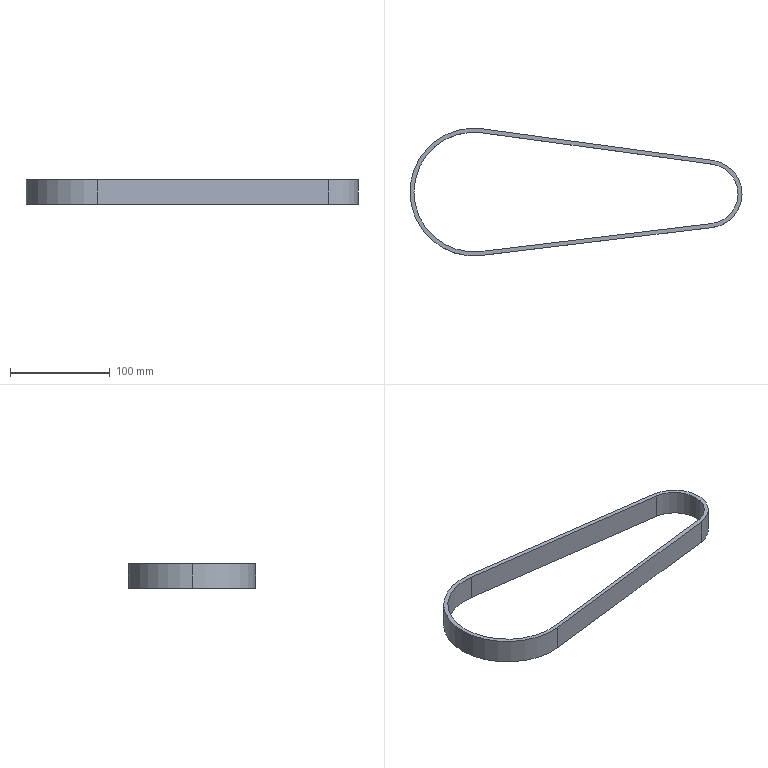Part | STEP file | Drive belt | 1 solid | 12 faces | box 332.993 x 128 x 25 mm | volume 76914 mm3 | cylinder 6 | plane 6 | commonest cylinder face diameters 120 x2 128 x2 60 x1 68 x1
STEP:
#1=CARTESIAN_POINT('',(-114.273,11.253,25.));
#2=VERTEX_POINT('',#1);
#3=CARTESIAN_POINT('',(-46.154,70.702,25.));
#4=VERTEX_POINT('',#3);
#5=CARTESIAN_POINT('',(-54.273,11.253,25.));
#6=DIRECTION('',(0.,0.,-1.));
#7=DIRECTION('',(-1.,0.,0.));
#8=AXIS2_PLACEMENT_3D('',#5,#6,#7);
#9=CIRCLE('',#8,60.);
#10=EDGE_CURVE('',#2,#4,#9,.T.);
#11=ORIENTED_EDGE('',*,*,#10,.F.);
#12=CARTESIAN_POINT('',(-114.273,11.253,0.));
#13=VERTEX_POINT('',#12);
#14=CARTESIAN_POINT('',(-114.273,11.253,25.));
#15=DIRECTION('',(0.,0.,-1.));
#16=VECTOR('',#15,1000.);
#17=LINE('',#14,#16);
#18=EDGE_CURVE('',#2,#13,#17,.T.);
#19=ORIENTED_EDGE('',*,*,#18,.T.);
#20=CARTESIAN_POINT('',(-46.154,70.702,0.));
#21=VERTEX_POINT('',#20);
#22=CARTESIAN_POINT('',(-54.273,11.253,0.));
#23=DIRECTION('',(0.,0.,1.));
#24=DIRECTION('',(-1.,0.,0.));
#25=AXIS2_PLACEMENT_3D('',#22,#23,#24);
#26=CIRCLE('',#25,60.);
#27=EDGE_CURVE('',#21,#13,#26,.T.);
#28=ORIENTED_EDGE('',*,*,#27,.F.);
#29=CARTESIAN_POINT('',(-46.154,70.702,25.));
#30=DIRECTION('',(0.,0.,-1.));
#31=VECTOR('',#30,1000.);
#32=LINE('',#29,#31);
#33=EDGE_CURVE('',#4,#21,#32,.T.);
#34=ORIENTED_EDGE('',*,*,#33,.F.);
#35=EDGE_LOOP('',(#11,#19,#28,#34));
#36=FACE_OUTER_BOUND('',#35,.T.);
#37=CARTESIAN_POINT('',(-54.273,11.253,25.));
#38=DIRECTION('',(0.,0.,-1.));
#39=DIRECTION('',(-1.,0.,0.));
#40=AXIS2_PLACEMENT_3D('',#37,#38,#39);
#41=CYLINDRICAL_SURFACE('',#40,60.);
#42=ADVANCED_FACE('',(#36),#41,.F.);
#43=CARTESIAN_POINT('',(-118.273,11.253,25.));
#44=VERTEX_POINT('',#43);
#45=CARTESIAN_POINT('',(-46.593,-52.284,25.));
#46=VERTEX_POINT('',#45);
#47=CARTESIAN_POINT('',(-54.273,11.253,25.));
#48=DIRECTION('',(0.,0.,1.));
#49=DIRECTION('',(-1.,0.,0.));
#50=AXIS2_PLACEMENT_3D('',#47,#48,#49);
#51=CIRCLE('',#50,64.);
#52=EDGE_CURVE('',#44,#46,#51,.T.);
#53=ORIENTED_EDGE('',*,*,#52,.F.);
#54=CARTESIAN_POINT('',(-118.273,11.253,0.));
#55=VERTEX_POINT('',#54);
#56=CARTESIAN_POINT('',(-118.273,11.253,25.));
#57=DIRECTION('',(0.,0.,-1.));
#58=VECTOR('',#57,1000.);
#59=LINE('',#56,#58);
#60=EDGE_CURVE('',#44,#55,#59,.T.);
#61=ORIENTED_EDGE('',*,*,#60,.T.);
#62=CARTESIAN_POINT('',(-46.593,-52.284,0.));
#63=VERTEX_POINT('',#62);
#64=CARTESIAN_POINT('',(-54.273,11.253,0.));
#65=DIRECTION('',(0.,0.,1.));
#66=DIRECTION('',(-1.,0.,0.));
#67=AXIS2_PLACEMENT_3D('',#64,#65,#66);
#68=CIRCLE('',#67,64.);
#69=EDGE_CURVE('',#55,#63,#68,.T.);
#70=ORIENTED_EDGE('',*,*,#69,.T.);
#71=CARTESIAN_POINT('',(-46.593,-52.284,25.));
#72=DIRECTION('',(0.,0.,1.));
#73=VECTOR('',#72,1000.);
#74=LINE('',#71,#73);
#75=EDGE_CURVE('',#63,#46,#74,.T.);
#76=ORIENTED_EDGE('',*,*,#75,.T.);
#77=EDGE_LOOP('',(#53,#61,#70,#76));
#78=FACE_OUTER_BOUND('',#77,.T.);
#79=CARTESIAN_POINT('',(-54.273,11.253,25.));
#80=DIRECTION('',(0.,0.,-1.));
#81=DIRECTION('',(-1.,0.,0.));
#82=AXIS2_PLACEMENT_3D('',#79,#80,#81);
#83=CYLINDRICAL_SURFACE('',#82,64.);
#84=ADVANCED_FACE('',(#78),#83,.T.);
#85=CARTESIAN_POINT('',(184.78,39.164,25.));
#86=VERTEX_POINT('',#85);
#87=CARTESIAN_POINT('',(-46.154,70.702,25.));
#88=DIRECTION('',(-0.9908,0.1353,0.));
#89=VECTOR('',#88,1000.);
#90=LINE('',#87,#89);
#91=EDGE_CURVE('',#86,#4,#90,.T.);
#92=ORIENTED_EDGE('',*,*,#91,.T.);
#93=ORIENTED_EDGE('',*,*,#33,.T.);
#94=CARTESIAN_POINT('',(184.78,39.164,0.));
#95=VERTEX_POINT('',#94);
#96=CARTESIAN_POINT('',(-46.154,70.702,0.));
#97=DIRECTION('',(0.9908,-0.1353,0.));
#98=VECTOR('',#97,1000.);
#99=LINE('',#96,#98);
#100=EDGE_CURVE('',#21,#95,#99,.T.);
#101=ORIENTED_EDGE('',*,*,#100,.T.);
#102=CARTESIAN_POINT('',(184.78,39.164,25.));
#103=DIRECTION('',(0.,0.,1.));
#104=VECTOR('',#103,1000.);
#105=LINE('',#102,#104);
#106=EDGE_CURVE('',#95,#86,#105,.T.);
#107=ORIENTED_EDGE('',*,*,#106,.T.);
#108=EDGE_LOOP('',(#92,#93,#101,#107));
#109=FACE_OUTER_BOUND('',#108,.T.);
#110=CARTESIAN_POINT('',(-46.154,70.702,25.));
#111=DIRECTION('',(-0.1353,-0.9908,0.));
#112=DIRECTION('',(0.9908,-0.1353,0.));
#113=AXIS2_PLACEMENT_3D('',#110,#111,#112);
#114=PLANE('',#113);
#115=ADVANCED_FACE('',(#109),#114,.T.);
#116=ORIENTED_EDGE('',*,*,#18,.F.);
#117=CARTESIAN_POINT('',(-47.073,-48.313,25.));
#118=VERTEX_POINT('',#117);
#119=CARTESIAN_POINT('',(-54.273,11.253,25.));
#120=DIRECTION('',(0.,0.,-1.));
#121=DIRECTION('',(-1.,0.,0.));
#122=AXIS2_PLACEMENT_3D('',#119,#120,#121);
#123=CIRCLE('',#122,60.);
#124=EDGE_CURVE('',#118,#2,#123,.T.);
#125=ORIENTED_EDGE('',*,*,#124,.F.);
#126=CARTESIAN_POINT('',(-47.073,-48.313,0.));
#127=VERTEX_POINT('',#126);
#128=CARTESIAN_POINT('',(-47.073,-48.313,25.));
#129=DIRECTION('',(0.,0.,1.));
#130=VECTOR('',#129,1000.);
#131=LINE('',#128,#130);
#132=EDGE_CURVE('',#127,#118,#131,.T.);
#133=ORIENTED_EDGE('',*,*,#132,.F.);
#134=CARTESIAN_POINT('',(-54.273,11.253,0.));
#135=DIRECTION('',(0.,0.,1.));
#136=DIRECTION('',(-1.,0.,0.));
#137=AXIS2_PLACEMENT_3D('',#134,#135,#136);
#138=CIRCLE('',#137,60.);
#139=EDGE_CURVE('',#13,#127,#138,.T.);
#140=ORIENTED_EDGE('',*,*,#139,.F.);
#141=EDGE_LOOP('',(#116,#125,#133,#140));
#142=FACE_OUTER_BOUND('',#141,.T.);
#143=CARTESIAN_POINT('',(-54.273,11.253,25.));
#144=DIRECTION('',(0.,0.,-1.));
#145=DIRECTION('',(-1.,0.,0.));
#146=AXIS2_PLACEMENT_3D('',#143,#144,#145);
#147=CYLINDRICAL_SURFACE('',#146,60.);
#148=ADVANCED_FACE('',(#142),#147,.F.);
#149=ORIENTED_EDGE('',*,*,#91,.F.);
#150=CARTESIAN_POINT('',(184.32,-20.344,25.));
#151=VERTEX_POINT('',#150);
#152=CARTESIAN_POINT('',(180.72,9.439,25.));
#153=DIRECTION('',(0.,0.,-1.));
#154=DIRECTION('',(-1.,0.,0.));
#155=AXIS2_PLACEMENT_3D('',#152,#153,#154);
#156=CIRCLE('',#155,30.);
#157=EDGE_CURVE('',#86,#151,#156,.T.);
#158=ORIENTED_EDGE('',*,*,#157,.T.);
#159=CARTESIAN_POINT('',(184.32,-20.344,25.));
#160=DIRECTION('',(-0.9928,-0.12,0.));
#161=VECTOR('',#160,1000.);
#162=LINE('',#159,#161);
#163=EDGE_CURVE('',#151,#118,#162,.T.);
#164=ORIENTED_EDGE('',*,*,#163,.T.);
#165=ORIENTED_EDGE('',*,*,#124,.T.);
#166=ORIENTED_EDGE('',*,*,#10,.T.);
#167=EDGE_LOOP('',(#149,#158,#164,#165,#166));
#168=FACE_BOUND('',#167,.T.);
#169=CARTESIAN_POINT('',(-45.613,74.665,25.));
#170=VERTEX_POINT('',#169);
#171=CARTESIAN_POINT('',(-54.273,11.253,25.));
#172=DIRECTION('',(0.,0.,1.));
#173=DIRECTION('',(-1.,0.,0.));
#174=AXIS2_PLACEMENT_3D('',#171,#172,#173);
#175=CIRCLE('',#174,64.);
#176=EDGE_CURVE('',#170,#44,#175,.T.);
#177=ORIENTED_EDGE('',*,*,#176,.T.);
#178=ORIENTED_EDGE('',*,*,#52,.T.);
#179=CARTESIAN_POINT('',(184.8,-24.315,25.));
#180=VERTEX_POINT('',#179);
#181=CARTESIAN_POINT('',(-46.593,-52.284,25.));
#182=DIRECTION('',(0.9928,0.12,0.));
#183=VECTOR('',#182,1000.);
#184=LINE('',#181,#183);
#185=EDGE_CURVE('',#46,#180,#184,.T.);
#186=ORIENTED_EDGE('',*,*,#185,.T.);
#187=CARTESIAN_POINT('',(185.321,43.127,25.));
#188=VERTEX_POINT('',#187);
#189=CARTESIAN_POINT('',(180.72,9.439,25.));
#190=DIRECTION('',(0.,0.,1.));
#191=DIRECTION('',(-1.,0.,0.));
#192=AXIS2_PLACEMENT_3D('',#189,#190,#191);
#193=CIRCLE('',#192,34.);
#194=EDGE_CURVE('',#180,#188,#193,.T.);
#195=ORIENTED_EDGE('',*,*,#194,.T.);
#196=CARTESIAN_POINT('',(185.321,43.127,25.));
#197=DIRECTION('',(-0.9908,0.1353,0.));
#198=VECTOR('',#197,1000.);
#199=LINE('',#196,#198);
#200=EDGE_CURVE('',#188,#170,#199,.T.);
#201=ORIENTED_EDGE('',*,*,#200,.T.);
#202=EDGE_LOOP('',(#177,#178,#186,#195,#201));
#203=FACE_OUTER_BOUND('',#202,.T.);
#204=CARTESIAN_POINT('',(180.72,9.439,25.));
#205=DIRECTION('',(0.,0.,1.));
#206=DIRECTION('',(1.,0.,0.));
#207=AXIS2_PLACEMENT_3D('',#204,#205,#206);
#208=PLANE('',#207);
#209=ADVANCED_FACE('',(#168,#203),#208,.T.);
#210=CARTESIAN_POINT('',(184.32,-20.344,0.));
#211=VERTEX_POINT('',#210);
#212=CARTESIAN_POINT('',(184.32,-20.344,25.));
#213=DIRECTION('',(0.,0.,-1.));
#214=VECTOR('',#213,1000.);
#215=LINE('',#212,#214);
#216=EDGE_CURVE('',#151,#211,#215,.T.);
#217=ORIENTED_EDGE('',*,*,#216,.F.);
#218=ORIENTED_EDGE('',*,*,#157,.F.);
#219=ORIENTED_EDGE('',*,*,#106,.F.);
#220=CARTESIAN_POINT('',(180.72,9.439,0.));
#221=DIRECTION('',(0.,0.,1.));
#222=DIRECTION('',(-1.,0.,0.));
#223=AXIS2_PLACEMENT_3D('',#220,#221,#222);
#224=CIRCLE('',#223,30.);
#225=EDGE_CURVE('',#211,#95,#224,.T.);
#226=ORIENTED_EDGE('',*,*,#225,.F.);
#227=EDGE_LOOP('',(#217,#218,#219,#226));
#228=FACE_OUTER_BOUND('',#227,.T.);
#229=CARTESIAN_POINT('',(180.72,9.439,25.));
#230=DIRECTION('',(0.,0.,-1.));
#231=DIRECTION('',(-1.,0.,0.));
#232=AXIS2_PLACEMENT_3D('',#229,#230,#231);
#233=CYLINDRICAL_SURFACE('',#232,30.);
#234=ADVANCED_FACE('',(#228),#233,.F.);
#235=ORIENTED_EDGE('',*,*,#27,.T.);
#236=ORIENTED_EDGE('',*,*,#139,.T.);
#237=CARTESIAN_POINT('',(184.32,-20.344,0.));
#238=DIRECTION('',(-0.9928,-0.12,0.));
#239=VECTOR('',#238,1000.);
#240=LINE('',#237,#239);
#241=EDGE_CURVE('',#211,#127,#240,.T.);
#242=ORIENTED_EDGE('',*,*,#241,.F.);
#243=ORIENTED_EDGE('',*,*,#225,.T.);
#244=ORIENTED_EDGE('',*,*,#100,.F.);
#245=EDGE_LOOP('',(#235,#236,#242,#243,#244));
#246=FACE_BOUND('',#245,.T.);
#247=CARTESIAN_POINT('',(184.8,-24.315,0.));
#248=VERTEX_POINT('',#247);
#249=CARTESIAN_POINT('',(-46.593,-52.284,0.));
#250=DIRECTION('',(0.9928,0.12,0.));
#251=VECTOR('',#250,1000.);
#252=LINE('',#249,#251);
#253=EDGE_CURVE('',#63,#248,#252,.T.);
#254=ORIENTED_EDGE('',*,*,#253,.F.);
#255=ORIENTED_EDGE('',*,*,#69,.F.);
#256=CARTESIAN_POINT('',(-45.613,74.665,0.));
#257=VERTEX_POINT('',#256);
#258=CARTESIAN_POINT('',(-54.273,11.253,0.));
#259=DIRECTION('',(0.,0.,1.));
#260=DIRECTION('',(-1.,0.,0.));
#261=AXIS2_PLACEMENT_3D('',#258,#259,#260);
#262=CIRCLE('',#261,64.);
#263=EDGE_CURVE('',#257,#55,#262,.T.);
#264=ORIENTED_EDGE('',*,*,#263,.F.);
#265=CARTESIAN_POINT('',(185.321,43.127,0.));
#266=VERTEX_POINT('',#265);
#267=CARTESIAN_POINT('',(185.321,43.127,0.));
#268=DIRECTION('',(-0.9908,0.1353,0.));
#269=VECTOR('',#268,1000.);
#270=LINE('',#267,#269);
#271=EDGE_CURVE('',#266,#257,#270,.T.);
#272=ORIENTED_EDGE('',*,*,#271,.F.);
#273=CARTESIAN_POINT('',(180.72,9.439,0.));
#274=DIRECTION('',(0.,0.,1.));
#275=DIRECTION('',(-1.,0.,0.));
#276=AXIS2_PLACEMENT_3D('',#273,#274,#275);
#277=CIRCLE('',#276,34.);
#278=EDGE_CURVE('',#248,#266,#277,.T.);
#279=ORIENTED_EDGE('',*,*,#278,.F.);
#280=EDGE_LOOP('',(#254,#255,#264,#272,#279));
#281=FACE_OUTER_BOUND('',#280,.T.);
#282=CARTESIAN_POINT('',(180.72,9.439,0.));
#283=DIRECTION('',(0.,0.,1.));
#284=DIRECTION('',(1.,0.,0.));
#285=AXIS2_PLACEMENT_3D('',#282,#283,#284);
#286=PLANE('',#285);
#287=ADVANCED_FACE('',(#246,#281),#286,.F.);
#288=ORIENTED_EDGE('',*,*,#163,.F.);
#289=ORIENTED_EDGE('',*,*,#216,.T.);
#290=ORIENTED_EDGE('',*,*,#241,.T.);
#291=ORIENTED_EDGE('',*,*,#132,.T.);
#292=EDGE_LOOP('',(#288,#289,#290,#291));
#293=FACE_OUTER_BOUND('',#292,.T.);
#294=CARTESIAN_POINT('',(-47.073,-48.313,25.));
#295=DIRECTION('',(-0.12,0.9928,0.));
#296=DIRECTION('',(-0.9928,-0.12,0.));
#297=AXIS2_PLACEMENT_3D('',#294,#295,#296);
#298=PLANE('',#297);
#299=ADVANCED_FACE('',(#293),#298,.T.);
#300=CARTESIAN_POINT('',(184.8,-24.315,25.));
#301=DIRECTION('',(0.,0.,-1.));
#302=VECTOR('',#301,1000.);
#303=LINE('',#300,#302);
#304=EDGE_CURVE('',#180,#248,#303,.T.);
#305=ORIENTED_EDGE('',*,*,#304,.F.);
#306=ORIENTED_EDGE('',*,*,#185,.F.);
#307=ORIENTED_EDGE('',*,*,#75,.F.);
#308=ORIENTED_EDGE('',*,*,#253,.T.);
#309=EDGE_LOOP('',(#305,#306,#307,#308));
#310=FACE_OUTER_BOUND('',#309,.T.);
#311=CARTESIAN_POINT('',(-46.593,-52.284,25.));
#312=DIRECTION('',(-0.12,0.9928,0.));
#313=DIRECTION('',(-0.9928,-0.12,0.));
#314=AXIS2_PLACEMENT_3D('',#311,#312,#313);
#315=PLANE('',#314);
#316=ADVANCED_FACE('',(#310),#315,.F.);
#317=ORIENTED_EDGE('',*,*,#60,.F.);
#318=ORIENTED_EDGE('',*,*,#176,.F.);
#319=CARTESIAN_POINT('',(-45.613,74.665,25.));
#320=DIRECTION('',(0.,0.,-1.));
#321=VECTOR('',#320,1000.);
#322=LINE('',#319,#321);
#323=EDGE_CURVE('',#170,#257,#322,.T.);
#324=ORIENTED_EDGE('',*,*,#323,.T.);
#325=ORIENTED_EDGE('',*,*,#263,.T.);
#326=EDGE_LOOP('',(#317,#318,#324,#325));
#327=FACE_OUTER_BOUND('',#326,.T.);
#328=CARTESIAN_POINT('',(-54.273,11.253,25.));
#329=DIRECTION('',(0.,0.,-1.));
#330=DIRECTION('',(-1.,0.,0.));
#331=AXIS2_PLACEMENT_3D('',#328,#329,#330);
#332=CYLINDRICAL_SURFACE('',#331,64.);
#333=ADVANCED_FACE('',(#327),#332,.T.);
#334=ORIENTED_EDGE('',*,*,#323,.F.);
#335=ORIENTED_EDGE('',*,*,#200,.F.);
#336=CARTESIAN_POINT('',(185.321,43.127,25.));
#337=DIRECTION('',(0.,0.,1.));
#338=VECTOR('',#337,1000.);
#339=LINE('',#336,#338);
#340=EDGE_CURVE('',#266,#188,#339,.T.);
#341=ORIENTED_EDGE('',*,*,#340,.F.);
#342=ORIENTED_EDGE('',*,*,#271,.T.);
#343=EDGE_LOOP('',(#334,#335,#341,#342));
#344=FACE_OUTER_BOUND('',#343,.T.);
#345=CARTESIAN_POINT('',(-45.613,74.665,25.));
#346=DIRECTION('',(-0.1353,-0.9908,0.));
#347=DIRECTION('',(0.9908,-0.1353,0.));
#348=AXIS2_PLACEMENT_3D('',#345,#346,#347);
#349=PLANE('',#348);
#350=ADVANCED_FACE('',(#344),#349,.F.);
#351=ORIENTED_EDGE('',*,*,#194,.F.);
#352=ORIENTED_EDGE('',*,*,#304,.T.);
#353=ORIENTED_EDGE('',*,*,#278,.T.);
#354=ORIENTED_EDGE('',*,*,#340,.T.);
#355=EDGE_LOOP('',(#351,#352,#353,#354));
#356=FACE_OUTER_BOUND('',#355,.T.);
#357=CARTESIAN_POINT('',(180.72,9.439,25.));
#358=DIRECTION('',(0.,0.,-1.));
#359=DIRECTION('',(-1.,0.,0.));
#360=AXIS2_PLACEMENT_3D('',#357,#358,#359);
#361=CYLINDRICAL_SURFACE('',#360,34.);
#362=ADVANCED_FACE('',(#356),#361,.T.);
#363=CLOSED_SHELL('',(#42,#84,#115,#148,#209,#234,#287,#299,#316,#333,#350,#362));
#364=MANIFOLD_SOLID_BREP('',#363);
#365=CARTESIAN_POINT('',(0.,0.,0.));
#366=DIRECTION('',(0.,0.,1.));
#367=DIRECTION('',(1.,0.,0.));
#368=AXIS2_PLACEMENT_3D('',#365,#366,#367);
#369=(LENGTH_UNIT()NAMED_UNIT(*)SI_UNIT(.MILLI.,.METRE.));
#370=UNCERTAINTY_MEASURE_WITH_UNIT(LENGTH_MEASURE(0.00001),#369,'','');
#371=(NAMED_UNIT(*)PLANE_ANGLE_UNIT()SI_UNIT($,.RADIAN.));
#372=(NAMED_UNIT(*)SI_UNIT($,.STERADIAN.)SOLID_ANGLE_UNIT());
#373=(GEOMETRIC_REPRESENTATION_CONTEXT(3)GLOBAL_UNCERTAINTY_ASSIGNED_CONTEXT((#370))GLOBAL_UNIT_ASSIGNED_CONTEXT((#369,#371,#372))REPRESENTATION_CONTEXT('',''));
#374=ADVANCED_BREP_SHAPE_REPRESENTATION('',(#364,#368),#373);